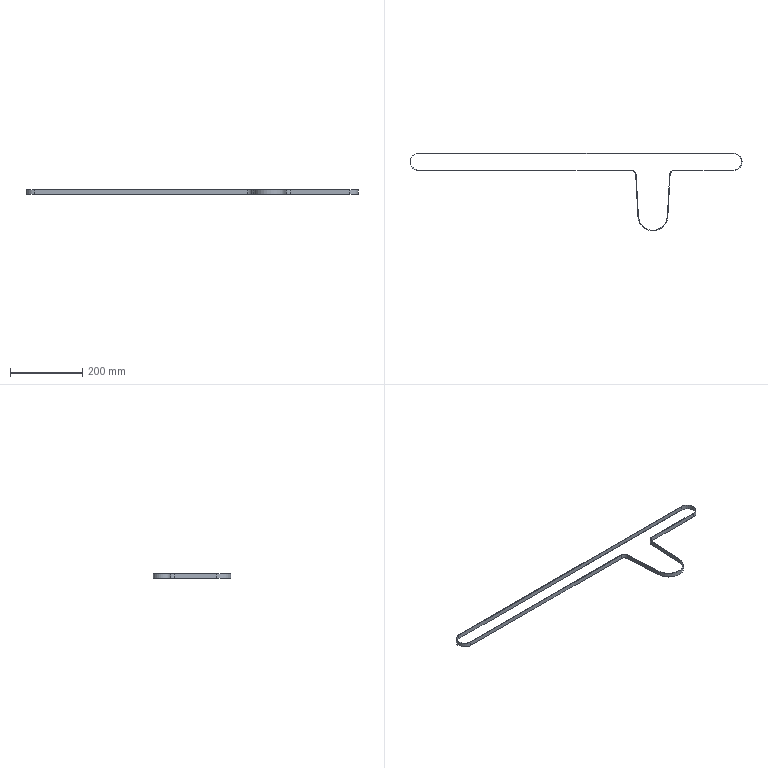Part | NX | features BREP 1 | 1 solid | 24 faces | box 917.4 x 214.1 x 12 mm | volume 31107 mm3 | cylinder 12 | plane 12 | commonest cylinder face diameters 45 x3 47.4 x3 25 x2 27.4 x2 80 x1 82.4 x1
STEP:
#1=CARTESIAN_POINT('',(764.214,8.857,-2.25));
#2=VERTEX_POINT('',#1);
#3=CARTESIAN_POINT('',(741.714,31.357,-2.25));
#4=VERTEX_POINT('',#3);
#5=CARTESIAN_POINT('',(741.714,8.857,-2.25));
#6=DIRECTION('',(0.,0.,1.));
#7=DIRECTION('',(-1.,0.,0.));
#8=AXIS2_PLACEMENT_3D('',#5,#6,#7);
#9=CIRCLE('',#8,22.5);
#10=EDGE_CURVE('',#2,#4,#9,.T.);
#11=ORIENTED_EDGE('',*,*,#10,.F.);
#12=CARTESIAN_POINT('',(764.214,8.857,9.75));
#13=VERTEX_POINT('',#12);
#14=CARTESIAN_POINT('',(764.214,8.857,-2.25));
#15=DIRECTION('',(0.,0.,1.));
#16=VECTOR('',#15,1000.);
#17=LINE('',#14,#16);
#18=EDGE_CURVE('',#2,#13,#17,.T.);
#19=ORIENTED_EDGE('',*,*,#18,.T.);
#20=CARTESIAN_POINT('',(741.714,31.357,9.75));
#21=VERTEX_POINT('',#20);
#22=CARTESIAN_POINT('',(741.714,8.857,9.75));
#23=DIRECTION('',(0.,0.,1.));
#24=DIRECTION('',(-1.,0.,0.));
#25=AXIS2_PLACEMENT_3D('',#22,#23,#24);
#26=CIRCLE('',#25,22.5);
#27=EDGE_CURVE('',#13,#21,#26,.T.);
#28=ORIENTED_EDGE('',*,*,#27,.T.);
#29=CARTESIAN_POINT('',(741.714,31.357,-2.25));
#30=DIRECTION('',(0.,0.,1.));
#31=VECTOR('',#30,1000.);
#32=LINE('',#29,#31);
#33=EDGE_CURVE('',#4,#21,#32,.T.);
#34=ORIENTED_EDGE('',*,*,#33,.F.);
#35=EDGE_LOOP('',(#11,#19,#28,#34));
#36=FACE_BOUND('',#35,.T.);
#37=CARTESIAN_POINT('',(741.714,8.857,-2.25));
#38=DIRECTION('',(0.,0.,1.));
#39=DIRECTION('',(1.,0.,0.));
#40=AXIS2_PLACEMENT_3D('',#37,#38,#39);
#41=CYLINDRICAL_SURFACE('',#40,22.5);
#42=ADVANCED_FACE('',(#36),#41,.F.);
#43=CARTESIAN_POINT('',(741.714,-14.843,-2.25));
#44=VERTEX_POINT('',#43);
#45=CARTESIAN_POINT('',(765.414,8.857,-2.25));
#46=VERTEX_POINT('',#45);
#47=CARTESIAN_POINT('',(741.714,8.857,-2.25));
#48=DIRECTION('',(0.,0.,1.));
#49=DIRECTION('',(1.,0.,0.));
#50=AXIS2_PLACEMENT_3D('',#47,#48,#49);
#51=CIRCLE('',#50,23.7);
#52=EDGE_CURVE('',#44,#46,#51,.T.);
#53=ORIENTED_EDGE('',*,*,#52,.T.);
#54=CARTESIAN_POINT('',(765.414,8.857,9.75));
#55=VERTEX_POINT('',#54);
#56=CARTESIAN_POINT('',(765.414,8.857,-2.25));
#57=DIRECTION('',(0.,0.,1.));
#58=VECTOR('',#57,1000.);
#59=LINE('',#56,#58);
#60=EDGE_CURVE('',#46,#55,#59,.T.);
#61=ORIENTED_EDGE('',*,*,#60,.T.);
#62=CARTESIAN_POINT('',(741.714,-14.843,9.75));
#63=VERTEX_POINT('',#62);
#64=CARTESIAN_POINT('',(741.714,8.857,9.75));
#65=DIRECTION('',(0.,0.,1.));
#66=DIRECTION('',(1.,0.,0.));
#67=AXIS2_PLACEMENT_3D('',#64,#65,#66);
#68=CIRCLE('',#67,23.7);
#69=EDGE_CURVE('',#63,#55,#68,.T.);
#70=ORIENTED_EDGE('',*,*,#69,.F.);
#71=CARTESIAN_POINT('',(741.714,-14.843,-2.25));
#72=DIRECTION('',(0.,0.,1.));
#73=VECTOR('',#72,1000.);
#74=LINE('',#71,#73);
#75=EDGE_CURVE('',#44,#63,#74,.T.);
#76=ORIENTED_EDGE('',*,*,#75,.F.);
#77=EDGE_LOOP('',(#53,#61,#70,#76));
#78=FACE_BOUND('',#77,.T.);
#79=CARTESIAN_POINT('',(741.714,8.857,-2.25));
#80=DIRECTION('',(0.,0.,1.));
#81=DIRECTION('',(1.,0.,0.));
#82=AXIS2_PLACEMENT_3D('',#79,#80,#81);
#83=CYLINDRICAL_SURFACE('',#82,23.7);
#84=ADVANCED_FACE('',(#78),#83,.T.);
#85=ORIENTED_EDGE('',*,*,#60,.F.);
#86=CARTESIAN_POINT('',(741.714,32.557,-2.25));
#87=VERTEX_POINT('',#86);
#88=CARTESIAN_POINT('',(741.714,8.857,-2.25));
#89=DIRECTION('',(0.,0.,1.));
#90=DIRECTION('',(1.,0.,0.));
#91=AXIS2_PLACEMENT_3D('',#88,#89,#90);
#92=CIRCLE('',#91,23.7);
#93=EDGE_CURVE('',#46,#87,#92,.T.);
#94=ORIENTED_EDGE('',*,*,#93,.T.);
#95=CARTESIAN_POINT('',(741.714,32.557,9.75));
#96=VERTEX_POINT('',#95);
#97=CARTESIAN_POINT('',(741.714,32.557,-2.25));
#98=DIRECTION('',(0.,0.,1.));
#99=VECTOR('',#98,1000.);
#100=LINE('',#97,#99);
#101=EDGE_CURVE('',#87,#96,#100,.T.);
#102=ORIENTED_EDGE('',*,*,#101,.T.);
#103=CARTESIAN_POINT('',(741.714,8.857,9.75));
#104=DIRECTION('',(0.,0.,1.));
#105=DIRECTION('',(1.,0.,0.));
#106=AXIS2_PLACEMENT_3D('',#103,#104,#105);
#107=CIRCLE('',#106,23.7);
#108=EDGE_CURVE('',#55,#96,#107,.T.);
#109=ORIENTED_EDGE('',*,*,#108,.F.);
#110=EDGE_LOOP('',(#85,#94,#102,#109));
#111=FACE_BOUND('',#110,.T.);
#112=CARTESIAN_POINT('',(741.714,8.857,-2.25));
#113=DIRECTION('',(0.,0.,1.));
#114=DIRECTION('',(1.,0.,0.));
#115=AXIS2_PLACEMENT_3D('',#112,#113,#114);
#116=CYLINDRICAL_SURFACE('',#115,23.7);
#117=ADVANCED_FACE('',(#111),#116,.T.);
#118=CARTESIAN_POINT('',(579.214,-14.843,9.75));
#119=VERTEX_POINT('',#118);
#120=CARTESIAN_POINT('',(579.214,-14.843,9.75));
#121=DIRECTION('',(1.,0.,0.));
#122=VECTOR('',#121,1000.);
#123=LINE('',#120,#122);
#124=EDGE_CURVE('',#119,#63,#123,.T.);
#125=ORIENTED_EDGE('',*,*,#124,.F.);
#126=CARTESIAN_POINT('',(579.214,-14.843,-2.25));
#127=VERTEX_POINT('',#126);
#128=CARTESIAN_POINT('',(579.214,-14.843,-2.25));
#129=DIRECTION('',(0.,0.,1.));
#130=VECTOR('',#129,1000.);
#131=LINE('',#128,#130);
#132=EDGE_CURVE('',#127,#119,#131,.T.);
#133=ORIENTED_EDGE('',*,*,#132,.F.);
#134=CARTESIAN_POINT('',(579.214,-14.843,-2.25));
#135=DIRECTION('',(1.,0.,0.));
#136=VECTOR('',#135,1000.);
#137=LINE('',#134,#136);
#138=EDGE_CURVE('',#127,#44,#137,.T.);
#139=ORIENTED_EDGE('',*,*,#138,.T.);
#140=ORIENTED_EDGE('',*,*,#75,.T.);
#141=EDGE_LOOP('',(#125,#133,#139,#140));
#142=FACE_BOUND('',#141,.T.);
#143=CARTESIAN_POINT('',(579.214,-14.843,-2.25));
#144=DIRECTION('',(0.,-1.,0.));
#145=DIRECTION('',(0.,0.,-1.));
#146=AXIS2_PLACEMENT_3D('',#143,#144,#145);
#147=PLANE('',#146);
#148=ADVANCED_FACE('',(#142),#147,.T.);
#149=CARTESIAN_POINT('',(566.733,-26.656,9.75));
#150=VERTEX_POINT('',#149);
#151=CARTESIAN_POINT('',(579.214,-27.343,9.75));
#152=DIRECTION('',(0.,0.,-1.));
#153=DIRECTION('',(-1.,0.,0.));
#154=AXIS2_PLACEMENT_3D('',#151,#152,#153);
#155=CIRCLE('',#154,12.5);
#156=EDGE_CURVE('',#150,#119,#155,.T.);
#157=ORIENTED_EDGE('',*,*,#156,.F.);
#158=CARTESIAN_POINT('',(566.733,-26.656,-2.25));
#159=VERTEX_POINT('',#158);
#160=CARTESIAN_POINT('',(566.733,-26.656,-2.25));
#161=DIRECTION('',(0.,0.,1.));
#162=VECTOR('',#161,1000.);
#163=LINE('',#160,#162);
#164=EDGE_CURVE('',#159,#150,#163,.T.);
#165=ORIENTED_EDGE('',*,*,#164,.F.);
#166=CARTESIAN_POINT('',(579.214,-27.343,-2.25));
#167=DIRECTION('',(0.,0.,-1.));
#168=DIRECTION('',(-1.,0.,0.));
#169=AXIS2_PLACEMENT_3D('',#166,#167,#168);
#170=CIRCLE('',#169,12.5);
#171=EDGE_CURVE('',#159,#127,#170,.T.);
#172=ORIENTED_EDGE('',*,*,#171,.T.);
#173=ORIENTED_EDGE('',*,*,#132,.T.);
#174=EDGE_LOOP('',(#157,#165,#172,#173));
#175=FACE_BOUND('',#174,.T.);
#176=CARTESIAN_POINT('',(579.214,-27.343,-2.25));
#177=DIRECTION('',(0.,0.,1.));
#178=DIRECTION('',(1.,0.,0.));
#179=AXIS2_PLACEMENT_3D('',#176,#177,#178);
#180=CYLINDRICAL_SURFACE('',#179,12.5);
#181=ADVANCED_FACE('',(#175),#180,.F.);
#182=CARTESIAN_POINT('',(560.352,-142.607,9.75));
#183=VERTEX_POINT('',#182);
#184=CARTESIAN_POINT('',(560.352,-142.607,9.75));
#185=DIRECTION('',(0.05495,0.9985,0.));
#186=VECTOR('',#185,1000.);
#187=LINE('',#184,#186);
#188=EDGE_CURVE('',#183,#150,#187,.T.);
#189=ORIENTED_EDGE('',*,*,#188,.F.);
#190=CARTESIAN_POINT('',(560.352,-142.607,-2.25));
#191=VERTEX_POINT('',#190);
#192=CARTESIAN_POINT('',(560.352,-142.607,-2.25));
#193=DIRECTION('',(0.,0.,1.));
#194=VECTOR('',#193,1000.);
#195=LINE('',#192,#194);
#196=EDGE_CURVE('',#191,#183,#195,.T.);
#197=ORIENTED_EDGE('',*,*,#196,.F.);
#198=CARTESIAN_POINT('',(560.352,-142.607,-2.25));
#199=DIRECTION('',(0.05495,0.9985,0.));
#200=VECTOR('',#199,1000.);
#201=LINE('',#198,#200);
#202=EDGE_CURVE('',#191,#159,#201,.T.);
#203=ORIENTED_EDGE('',*,*,#202,.T.);
#204=ORIENTED_EDGE('',*,*,#164,.T.);
#205=EDGE_LOOP('',(#189,#197,#203,#204));
#206=FACE_BOUND('',#205,.T.);
#207=CARTESIAN_POINT('',(560.352,-142.607,-2.25));
#208=DIRECTION('',(0.9985,-0.05495,0.));
#209=DIRECTION('',(0.,0.,-1.));
#210=AXIS2_PLACEMENT_3D('',#207,#208,#209);
#211=PLANE('',#210);
#212=ADVANCED_FACE('',(#206),#211,.T.);
#213=CARTESIAN_POINT('',(478.077,-142.607,9.75));
#214=VERTEX_POINT('',#213);
#215=CARTESIAN_POINT('',(519.214,-140.343,9.75));
#216=DIRECTION('',(0.,0.,1.));
#217=DIRECTION('',(1.,0.,0.));
#218=AXIS2_PLACEMENT_3D('',#215,#216,#217);
#219=CIRCLE('',#218,41.2);
#220=EDGE_CURVE('',#214,#183,#219,.T.);
#221=ORIENTED_EDGE('',*,*,#220,.F.);
#222=CARTESIAN_POINT('',(478.077,-142.607,-2.25));
#223=VERTEX_POINT('',#222);
#224=CARTESIAN_POINT('',(478.077,-142.607,-2.25));
#225=DIRECTION('',(0.,0.,1.));
#226=VECTOR('',#225,1000.);
#227=LINE('',#224,#226);
#228=EDGE_CURVE('',#223,#214,#227,.T.);
#229=ORIENTED_EDGE('',*,*,#228,.F.);
#230=CARTESIAN_POINT('',(519.214,-140.343,-2.25));
#231=DIRECTION('',(0.,0.,1.));
#232=DIRECTION('',(1.,0.,0.));
#233=AXIS2_PLACEMENT_3D('',#230,#231,#232);
#234=CIRCLE('',#233,41.2);
#235=EDGE_CURVE('',#223,#191,#234,.T.);
#236=ORIENTED_EDGE('',*,*,#235,.T.);
#237=ORIENTED_EDGE('',*,*,#196,.T.);
#238=EDGE_LOOP('',(#221,#229,#236,#237));
#239=FACE_BOUND('',#238,.T.);
#240=CARTESIAN_POINT('',(519.214,-140.343,-2.25));
#241=DIRECTION('',(0.,0.,1.));
#242=DIRECTION('',(1.,0.,0.));
#243=AXIS2_PLACEMENT_3D('',#240,#241,#242);
#244=CYLINDRICAL_SURFACE('',#243,41.2);
#245=ADVANCED_FACE('',(#239),#244,.T.);
#246=CARTESIAN_POINT('',(471.695,-26.656,9.75));
#247=VERTEX_POINT('',#246);
#248=CARTESIAN_POINT('',(471.695,-26.656,9.75));
#249=DIRECTION('',(0.05495,-0.9985,0.));
#250=VECTOR('',#249,1000.);
#251=LINE('',#248,#250);
#252=EDGE_CURVE('',#247,#214,#251,.T.);
#253=ORIENTED_EDGE('',*,*,#252,.F.);
#254=CARTESIAN_POINT('',(471.695,-26.656,-2.25));
#255=VERTEX_POINT('',#254);
#256=CARTESIAN_POINT('',(471.695,-26.656,-2.25));
#257=DIRECTION('',(0.,0.,1.));
#258=VECTOR('',#257,1000.);
#259=LINE('',#256,#258);
#260=EDGE_CURVE('',#255,#247,#259,.T.);
#261=ORIENTED_EDGE('',*,*,#260,.F.);
#262=CARTESIAN_POINT('',(471.695,-26.656,-2.25));
#263=DIRECTION('',(0.05495,-0.9985,0.));
#264=VECTOR('',#263,1000.);
#265=LINE('',#262,#264);
#266=EDGE_CURVE('',#255,#223,#265,.T.);
#267=ORIENTED_EDGE('',*,*,#266,.T.);
#268=ORIENTED_EDGE('',*,*,#228,.T.);
#269=EDGE_LOOP('',(#253,#261,#267,#268));
#270=FACE_BOUND('',#269,.T.);
#271=CARTESIAN_POINT('',(471.695,-26.656,-2.25));
#272=DIRECTION('',(-0.9985,-0.05495,0.));
#273=DIRECTION('',(-0.05495,0.9985,0.));
#274=AXIS2_PLACEMENT_3D('',#271,#272,#273);
#275=PLANE('',#274);
#276=ADVANCED_FACE('',(#270),#275,.T.);
#277=CARTESIAN_POINT('',(459.214,-14.843,9.75));
#278=VERTEX_POINT('',#277);
#279=CARTESIAN_POINT('',(459.214,-27.343,9.75));
#280=DIRECTION('',(0.,0.,-1.));
#281=DIRECTION('',(-1.,0.,0.));
#282=AXIS2_PLACEMENT_3D('',#279,#280,#281);
#283=CIRCLE('',#282,12.5);
#284=EDGE_CURVE('',#278,#247,#283,.T.);
#285=ORIENTED_EDGE('',*,*,#284,.F.);
#286=CARTESIAN_POINT('',(459.214,-14.843,-2.25));
#287=VERTEX_POINT('',#286);
#288=CARTESIAN_POINT('',(459.214,-14.843,-2.25));
#289=DIRECTION('',(0.,0.,1.));
#290=VECTOR('',#289,1000.);
#291=LINE('',#288,#290);
#292=EDGE_CURVE('',#287,#278,#291,.T.);
#293=ORIENTED_EDGE('',*,*,#292,.F.);
#294=CARTESIAN_POINT('',(459.214,-27.343,-2.25));
#295=DIRECTION('',(0.,0.,-1.));
#296=DIRECTION('',(-1.,0.,0.));
#297=AXIS2_PLACEMENT_3D('',#294,#295,#296);
#298=CIRCLE('',#297,12.5);
#299=EDGE_CURVE('',#287,#255,#298,.T.);
#300=ORIENTED_EDGE('',*,*,#299,.T.);
#301=ORIENTED_EDGE('',*,*,#260,.T.);
#302=EDGE_LOOP('',(#285,#293,#300,#301));
#303=FACE_BOUND('',#302,.T.);
#304=CARTESIAN_POINT('',(459.214,-27.343,-2.25));
#305=DIRECTION('',(0.,0.,1.));
#306=DIRECTION('',(1.,0.,0.));
#307=AXIS2_PLACEMENT_3D('',#304,#305,#306);
#308=CYLINDRICAL_SURFACE('',#307,12.5);
#309=ADVANCED_FACE('',(#303),#308,.F.);
#310=CARTESIAN_POINT('',(-128.286,-14.843,9.75));
#311=VERTEX_POINT('',#310);
#312=CARTESIAN_POINT('',(-128.286,-14.843,9.75));
#313=DIRECTION('',(1.,0.,0.));
#314=VECTOR('',#313,1000.);
#315=LINE('',#312,#314);
#316=EDGE_CURVE('',#311,#278,#315,.T.);
#317=ORIENTED_EDGE('',*,*,#316,.F.);
#318=CARTESIAN_POINT('',(-128.286,-14.843,-2.25));
#319=VERTEX_POINT('',#318);
#320=CARTESIAN_POINT('',(-128.286,-14.843,-2.25));
#321=DIRECTION('',(0.,0.,1.));
#322=VECTOR('',#321,1000.);
#323=LINE('',#320,#322);
#324=EDGE_CURVE('',#319,#311,#323,.T.);
#325=ORIENTED_EDGE('',*,*,#324,.F.);
#326=CARTESIAN_POINT('',(-128.286,-14.843,-2.25));
#327=DIRECTION('',(1.,0.,0.));
#328=VECTOR('',#327,1000.);
#329=LINE('',#326,#328);
#330=EDGE_CURVE('',#319,#287,#329,.T.);
#331=ORIENTED_EDGE('',*,*,#330,.T.);
#332=ORIENTED_EDGE('',*,*,#292,.T.);
#333=EDGE_LOOP('',(#317,#325,#331,#332));
#334=FACE_BOUND('',#333,.T.);
#335=CARTESIAN_POINT('',(-128.286,-14.843,-2.25));
#336=DIRECTION('',(0.,-1.,0.));
#337=DIRECTION('',(-1.,0.,0.));
#338=AXIS2_PLACEMENT_3D('',#335,#336,#337);
#339=PLANE('',#338);
#340=ADVANCED_FACE('',(#334),#339,.T.);
#341=CARTESIAN_POINT('',(-128.286,32.557,9.75));
#342=VERTEX_POINT('',#341);
#343=CARTESIAN_POINT('',(-128.286,8.857,9.75));
#344=DIRECTION('',(0.,0.,1.));
#345=DIRECTION('',(1.,0.,0.));
#346=AXIS2_PLACEMENT_3D('',#343,#344,#345);
#347=CIRCLE('',#346,23.7);
#348=EDGE_CURVE('',#342,#311,#347,.T.);
#349=ORIENTED_EDGE('',*,*,#348,.F.);
#350=CARTESIAN_POINT('',(-128.286,32.557,-2.25));
#351=VERTEX_POINT('',#350);
#352=CARTESIAN_POINT('',(-128.286,32.557,-2.25));
#353=DIRECTION('',(0.,0.,1.));
#354=VECTOR('',#353,1000.);
#355=LINE('',#352,#354);
#356=EDGE_CURVE('',#351,#342,#355,.T.);
#357=ORIENTED_EDGE('',*,*,#356,.F.);
#358=CARTESIAN_POINT('',(-128.286,8.857,-2.25));
#359=DIRECTION('',(0.,0.,1.));
#360=DIRECTION('',(1.,0.,0.));
#361=AXIS2_PLACEMENT_3D('',#358,#359,#360);
#362=CIRCLE('',#361,23.7);
#363=EDGE_CURVE('',#351,#319,#362,.T.);
#364=ORIENTED_EDGE('',*,*,#363,.T.);
#365=ORIENTED_EDGE('',*,*,#324,.T.);
#366=EDGE_LOOP('',(#349,#357,#364,#365));
#367=FACE_BOUND('',#366,.T.);
#368=CARTESIAN_POINT('',(-128.286,8.857,-2.25));
#369=DIRECTION('',(0.,0.,1.));
#370=DIRECTION('',(1.,0.,0.));
#371=AXIS2_PLACEMENT_3D('',#368,#369,#370);
#372=CYLINDRICAL_SURFACE('',#371,23.7);
#373=ADVANCED_FACE('',(#367),#372,.T.);
#374=CARTESIAN_POINT('',(741.714,32.557,9.75));
#375=DIRECTION('',(-1.,0.,0.));
#376=VECTOR('',#375,1000.);
#377=LINE('',#374,#376);
#378=EDGE_CURVE('',#96,#342,#377,.T.);
#379=ORIENTED_EDGE('',*,*,#378,.F.);
#380=ORIENTED_EDGE('',*,*,#101,.F.);
#381=CARTESIAN_POINT('',(741.714,32.557,-2.25));
#382=DIRECTION('',(-1.,0.,0.));
#383=VECTOR('',#382,1000.);
#384=LINE('',#381,#383);
#385=EDGE_CURVE('',#87,#351,#384,.T.);
#386=ORIENTED_EDGE('',*,*,#385,.T.);
#387=ORIENTED_EDGE('',*,*,#356,.T.);
#388=EDGE_LOOP('',(#379,#380,#386,#387));
#389=FACE_BOUND('',#388,.T.);
#390=CARTESIAN_POINT('',(741.714,32.557,-2.25));
#391=DIRECTION('',(0.,1.,0.));
#392=DIRECTION('',(1.,0.,0.));
#393=AXIS2_PLACEMENT_3D('',#390,#391,#392);
#394=PLANE('',#393);
#395=ADVANCED_FACE('',(#389),#394,.T.);
#396=ORIENTED_EDGE('',*,*,#52,.F.);
#397=ORIENTED_EDGE('',*,*,#138,.F.);
#398=ORIENTED_EDGE('',*,*,#171,.F.);
#399=ORIENTED_EDGE('',*,*,#202,.F.);
#400=ORIENTED_EDGE('',*,*,#235,.F.);
#401=ORIENTED_EDGE('',*,*,#266,.F.);
#402=ORIENTED_EDGE('',*,*,#299,.F.);
#403=ORIENTED_EDGE('',*,*,#330,.F.);
#404=ORIENTED_EDGE('',*,*,#363,.F.);
#405=ORIENTED_EDGE('',*,*,#385,.F.);
#406=ORIENTED_EDGE('',*,*,#93,.F.);
#407=EDGE_LOOP('',(#396,#397,#398,#399,#400,#401,#402,#403,#404,#405,#406));
#408=FACE_BOUND('',#407,.T.);
#409=CARTESIAN_POINT('',(472.894,-26.59,-2.25));
#410=VERTEX_POINT('',#409);
#411=CARTESIAN_POINT('',(479.275,-142.541,-2.25));
#412=VERTEX_POINT('',#411);
#413=CARTESIAN_POINT('',(479.275,-142.541,-2.25));
#414=DIRECTION('',(0.05495,-0.9985,0.));
#415=VECTOR('',#414,1000.);
#416=LINE('',#413,#415);
#417=EDGE_CURVE('',#410,#412,#416,.T.);
#418=ORIENTED_EDGE('',*,*,#417,.T.);
#419=CARTESIAN_POINT('',(559.154,-142.541,-2.25));
#420=VERTEX_POINT('',#419);
#421=CARTESIAN_POINT('',(519.214,-140.343,-2.25));
#422=DIRECTION('',(0.,0.,1.));
#423=DIRECTION('',(-1.,0.,0.));
#424=AXIS2_PLACEMENT_3D('',#421,#422,#423);
#425=CIRCLE('',#424,40.);
#426=EDGE_CURVE('',#412,#420,#425,.T.);
#427=ORIENTED_EDGE('',*,*,#426,.T.);
#428=CARTESIAN_POINT('',(565.535,-26.59,-2.25));
#429=VERTEX_POINT('',#428);
#430=CARTESIAN_POINT('',(565.535,-26.59,-2.25));
#431=DIRECTION('',(0.05495,0.9985,0.));
#432=VECTOR('',#431,1000.);
#433=LINE('',#430,#432);
#434=EDGE_CURVE('',#420,#429,#433,.T.);
#435=ORIENTED_EDGE('',*,*,#434,.T.);
#436=CARTESIAN_POINT('',(579.214,-13.643,-2.25));
#437=VERTEX_POINT('',#436);
#438=CARTESIAN_POINT('',(579.214,-27.343,-2.25));
#439=DIRECTION('',(0.,0.,-1.));
#440=DIRECTION('',(1.,0.,0.));
#441=AXIS2_PLACEMENT_3D('',#438,#439,#440);
#442=CIRCLE('',#441,13.7);
#443=EDGE_CURVE('',#429,#437,#442,.T.);
#444=ORIENTED_EDGE('',*,*,#443,.T.);
#445=CARTESIAN_POINT('',(741.714,-13.643,-2.25));
#446=VERTEX_POINT('',#445);
#447=CARTESIAN_POINT('',(741.714,-13.643,-2.25));
#448=DIRECTION('',(1.,0.,0.));
#449=VECTOR('',#448,1000.);
#450=LINE('',#447,#449);
#451=EDGE_CURVE('',#437,#446,#450,.T.);
#452=ORIENTED_EDGE('',*,*,#451,.T.);
#453=CARTESIAN_POINT('',(741.714,8.857,-2.25));
#454=DIRECTION('',(0.,0.,1.));
#455=DIRECTION('',(-1.,0.,0.));
#456=AXIS2_PLACEMENT_3D('',#453,#454,#455);
#457=CIRCLE('',#456,22.5);
#458=EDGE_CURVE('',#446,#2,#457,.T.);
#459=ORIENTED_EDGE('',*,*,#458,.T.);
#460=ORIENTED_EDGE('',*,*,#10,.T.);
#461=CARTESIAN_POINT('',(-128.286,31.357,-2.25));
#462=VERTEX_POINT('',#461);
#463=CARTESIAN_POINT('',(-128.286,31.357,-2.25));
#464=DIRECTION('',(-1.,0.,0.));
#465=VECTOR('',#464,1000.);
#466=LINE('',#463,#465);
#467=EDGE_CURVE('',#4,#462,#466,.T.);
#468=ORIENTED_EDGE('',*,*,#467,.T.);
#469=CARTESIAN_POINT('',(-128.286,-13.643,-2.25));
#470=VERTEX_POINT('',#469);
#471=CARTESIAN_POINT('',(-128.286,8.857,-2.25));
#472=DIRECTION('',(0.,0.,1.));
#473=DIRECTION('',(-1.,0.,0.));
#474=AXIS2_PLACEMENT_3D('',#471,#472,#473);
#475=CIRCLE('',#474,22.5);
#476=EDGE_CURVE('',#462,#470,#475,.T.);
#477=ORIENTED_EDGE('',*,*,#476,.T.);
#478=CARTESIAN_POINT('',(459.214,-13.643,-2.25));
#479=VERTEX_POINT('',#478);
#480=CARTESIAN_POINT('',(459.214,-13.643,-2.25));
#481=DIRECTION('',(1.,0.,0.));
#482=VECTOR('',#481,1000.);
#483=LINE('',#480,#482);
#484=EDGE_CURVE('',#470,#479,#483,.T.);
#485=ORIENTED_EDGE('',*,*,#484,.T.);
#486=CARTESIAN_POINT('',(459.214,-27.343,-2.25));
#487=DIRECTION('',(0.,0.,-1.));
#488=DIRECTION('',(1.,0.,0.));
#489=AXIS2_PLACEMENT_3D('',#486,#487,#488);
#490=CIRCLE('',#489,13.7);
#491=EDGE_CURVE('',#479,#410,#490,.T.);
#492=ORIENTED_EDGE('',*,*,#491,.T.);
#493=EDGE_LOOP('',(#418,#427,#435,#444,#452,#459,#460,#468,#477,#485,#492));
#494=FACE_BOUND('',#493,.T.);
#495=CARTESIAN_POINT('',(741.714,8.857,-2.25));
#496=DIRECTION('',(0.,0.,1.));
#497=DIRECTION('',(1.,0.,0.));
#498=AXIS2_PLACEMENT_3D('',#495,#496,#497);
#499=PLANE('',#498);
#500=ADVANCED_FACE('',(#408,#494),#499,.F.);
#501=ORIENTED_EDGE('',*,*,#69,.T.);
#502=ORIENTED_EDGE('',*,*,#108,.T.);
#503=ORIENTED_EDGE('',*,*,#378,.T.);
#504=ORIENTED_EDGE('',*,*,#348,.T.);
#505=ORIENTED_EDGE('',*,*,#316,.T.);
#506=ORIENTED_EDGE('',*,*,#284,.T.);
#507=ORIENTED_EDGE('',*,*,#252,.T.);
#508=ORIENTED_EDGE('',*,*,#220,.T.);
#509=ORIENTED_EDGE('',*,*,#188,.T.);
#510=ORIENTED_EDGE('',*,*,#156,.T.);
#511=ORIENTED_EDGE('',*,*,#124,.T.);
#512=EDGE_LOOP('',(#501,#502,#503,#504,#505,#506,#507,#508,#509,#510,#511));
#513=FACE_BOUND('',#512,.T.);
#514=CARTESIAN_POINT('',(479.275,-142.541,9.75));
#515=VERTEX_POINT('',#514);
#516=CARTESIAN_POINT('',(559.154,-142.541,9.75));
#517=VERTEX_POINT('',#516);
#518=CARTESIAN_POINT('',(519.214,-140.343,9.75));
#519=DIRECTION('',(0.,0.,1.));
#520=DIRECTION('',(-1.,0.,0.));
#521=AXIS2_PLACEMENT_3D('',#518,#519,#520);
#522=CIRCLE('',#521,40.);
#523=EDGE_CURVE('',#515,#517,#522,.T.);
#524=ORIENTED_EDGE('',*,*,#523,.F.);
#525=CARTESIAN_POINT('',(472.894,-26.59,9.75));
#526=VERTEX_POINT('',#525);
#527=CARTESIAN_POINT('',(479.275,-142.541,9.75));
#528=DIRECTION('',(0.05495,-0.9985,0.));
#529=VECTOR('',#528,1000.);
#530=LINE('',#527,#529);
#531=EDGE_CURVE('',#526,#515,#530,.T.);
#532=ORIENTED_EDGE('',*,*,#531,.F.);
#533=CARTESIAN_POINT('',(459.214,-13.643,9.75));
#534=VERTEX_POINT('',#533);
#535=CARTESIAN_POINT('',(459.214,-27.343,9.75));
#536=DIRECTION('',(0.,0.,-1.));
#537=DIRECTION('',(1.,0.,0.));
#538=AXIS2_PLACEMENT_3D('',#535,#536,#537);
#539=CIRCLE('',#538,13.7);
#540=EDGE_CURVE('',#534,#526,#539,.T.);
#541=ORIENTED_EDGE('',*,*,#540,.F.);
#542=CARTESIAN_POINT('',(-128.286,-13.643,9.75));
#543=VERTEX_POINT('',#542);
#544=CARTESIAN_POINT('',(459.214,-13.643,9.75));
#545=DIRECTION('',(1.,0.,0.));
#546=VECTOR('',#545,1000.);
#547=LINE('',#544,#546);
#548=EDGE_CURVE('',#543,#534,#547,.T.);
#549=ORIENTED_EDGE('',*,*,#548,.F.);
#550=CARTESIAN_POINT('',(-128.286,31.357,9.75));
#551=VERTEX_POINT('',#550);
#552=CARTESIAN_POINT('',(-128.286,8.857,9.75));
#553=DIRECTION('',(0.,0.,1.));
#554=DIRECTION('',(-1.,0.,0.));
#555=AXIS2_PLACEMENT_3D('',#552,#553,#554);
#556=CIRCLE('',#555,22.5);
#557=EDGE_CURVE('',#551,#543,#556,.T.);
#558=ORIENTED_EDGE('',*,*,#557,.F.);
#559=CARTESIAN_POINT('',(-128.286,31.357,9.75));
#560=DIRECTION('',(-1.,0.,0.));
#561=VECTOR('',#560,1000.);
#562=LINE('',#559,#561);
#563=EDGE_CURVE('',#21,#551,#562,.T.);
#564=ORIENTED_EDGE('',*,*,#563,.F.);
#565=ORIENTED_EDGE('',*,*,#27,.F.);
#566=CARTESIAN_POINT('',(741.714,-13.643,9.75));
#567=VERTEX_POINT('',#566);
#568=CARTESIAN_POINT('',(741.714,8.857,9.75));
#569=DIRECTION('',(0.,0.,1.));
#570=DIRECTION('',(-1.,0.,0.));
#571=AXIS2_PLACEMENT_3D('',#568,#569,#570);
#572=CIRCLE('',#571,22.5);
#573=EDGE_CURVE('',#567,#13,#572,.T.);
#574=ORIENTED_EDGE('',*,*,#573,.F.);
#575=CARTESIAN_POINT('',(579.214,-13.643,9.75));
#576=VERTEX_POINT('',#575);
#577=CARTESIAN_POINT('',(741.714,-13.643,9.75));
#578=DIRECTION('',(1.,0.,0.));
#579=VECTOR('',#578,1000.);
#580=LINE('',#577,#579);
#581=EDGE_CURVE('',#576,#567,#580,.T.);
#582=ORIENTED_EDGE('',*,*,#581,.F.);
#583=CARTESIAN_POINT('',(565.535,-26.59,9.75));
#584=VERTEX_POINT('',#583);
#585=CARTESIAN_POINT('',(579.214,-27.343,9.75));
#586=DIRECTION('',(0.,0.,-1.));
#587=DIRECTION('',(1.,0.,0.));
#588=AXIS2_PLACEMENT_3D('',#585,#586,#587);
#589=CIRCLE('',#588,13.7);
#590=EDGE_CURVE('',#584,#576,#589,.T.);
#591=ORIENTED_EDGE('',*,*,#590,.F.);
#592=CARTESIAN_POINT('',(565.535,-26.59,9.75));
#593=DIRECTION('',(0.05495,0.9985,0.));
#594=VECTOR('',#593,1000.);
#595=LINE('',#592,#594);
#596=EDGE_CURVE('',#517,#584,#595,.T.);
#597=ORIENTED_EDGE('',*,*,#596,.F.);
#598=EDGE_LOOP('',(#524,#532,#541,#549,#558,#564,#565,#574,#582,#591,#597));
#599=FACE_BOUND('',#598,.T.);
#600=CARTESIAN_POINT('',(741.714,8.857,9.75));
#601=DIRECTION('',(0.,0.,1.));
#602=DIRECTION('',(1.,0.,0.));
#603=AXIS2_PLACEMENT_3D('',#600,#601,#602);
#604=PLANE('',#603);
#605=ADVANCED_FACE('',(#513,#599),#604,.T.);
#606=ORIENTED_EDGE('',*,*,#523,.T.);
#607=CARTESIAN_POINT('',(559.154,-142.541,-2.25));
#608=DIRECTION('',(0.,0.,1.));
#609=VECTOR('',#608,1000.);
#610=LINE('',#607,#609);
#611=EDGE_CURVE('',#420,#517,#610,.T.);
#612=ORIENTED_EDGE('',*,*,#611,.F.);
#613=ORIENTED_EDGE('',*,*,#426,.F.);
#614=CARTESIAN_POINT('',(479.275,-142.541,-2.25));
#615=DIRECTION('',(0.,0.,1.));
#616=VECTOR('',#615,1000.);
#617=LINE('',#614,#616);
#618=EDGE_CURVE('',#412,#515,#617,.T.);
#619=ORIENTED_EDGE('',*,*,#618,.T.);
#620=EDGE_LOOP('',(#606,#612,#613,#619));
#621=FACE_BOUND('',#620,.T.);
#622=CARTESIAN_POINT('',(519.214,-140.343,-2.25));
#623=DIRECTION('',(0.,0.,1.));
#624=DIRECTION('',(1.,0.,0.));
#625=AXIS2_PLACEMENT_3D('',#622,#623,#624);
#626=CYLINDRICAL_SURFACE('',#625,40.);
#627=ADVANCED_FACE('',(#621),#626,.F.);
#628=ORIENTED_EDGE('',*,*,#531,.T.);
#629=ORIENTED_EDGE('',*,*,#618,.F.);
#630=ORIENTED_EDGE('',*,*,#417,.F.);
#631=CARTESIAN_POINT('',(472.894,-26.59,-2.25));
#632=DIRECTION('',(0.,0.,1.));
#633=VECTOR('',#632,1000.);
#634=LINE('',#631,#633);
#635=EDGE_CURVE('',#410,#526,#634,.T.);
#636=ORIENTED_EDGE('',*,*,#635,.T.);
#637=EDGE_LOOP('',(#628,#629,#630,#636));
#638=FACE_BOUND('',#637,.T.);
#639=CARTESIAN_POINT('',(479.275,-142.541,-2.25));
#640=DIRECTION('',(-0.9985,-0.05495,0.));
#641=DIRECTION('',(-0.05495,0.9985,0.));
#642=AXIS2_PLACEMENT_3D('',#639,#640,#641);
#643=PLANE('',#642);
#644=ADVANCED_FACE('',(#638),#643,.F.);
#645=ORIENTED_EDGE('',*,*,#540,.T.);
#646=ORIENTED_EDGE('',*,*,#635,.F.);
#647=ORIENTED_EDGE('',*,*,#491,.F.);
#648=CARTESIAN_POINT('',(459.214,-13.643,-2.25));
#649=DIRECTION('',(0.,0.,1.));
#650=VECTOR('',#649,1000.);
#651=LINE('',#648,#650);
#652=EDGE_CURVE('',#479,#534,#651,.T.);
#653=ORIENTED_EDGE('',*,*,#652,.T.);
#654=EDGE_LOOP('',(#645,#646,#647,#653));
#655=FACE_BOUND('',#654,.T.);
#656=CARTESIAN_POINT('',(459.214,-27.343,-2.25));
#657=DIRECTION('',(0.,0.,1.));
#658=DIRECTION('',(1.,0.,0.));
#659=AXIS2_PLACEMENT_3D('',#656,#657,#658);
#660=CYLINDRICAL_SURFACE('',#659,13.7);
#661=ADVANCED_FACE('',(#655),#660,.T.);
#662=ORIENTED_EDGE('',*,*,#548,.T.);
#663=ORIENTED_EDGE('',*,*,#652,.F.);
#664=ORIENTED_EDGE('',*,*,#484,.F.);
#665=CARTESIAN_POINT('',(-128.286,-13.643,-2.25));
#666=DIRECTION('',(0.,0.,1.));
#667=VECTOR('',#666,1000.);
#668=LINE('',#665,#667);
#669=EDGE_CURVE('',#470,#543,#668,.T.);
#670=ORIENTED_EDGE('',*,*,#669,.T.);
#671=EDGE_LOOP('',(#662,#663,#664,#670));
#672=FACE_BOUND('',#671,.T.);
#673=CARTESIAN_POINT('',(459.214,-13.643,-2.25));
#674=DIRECTION('',(0.,-1.,0.));
#675=DIRECTION('',(0.,0.,-1.));
#676=AXIS2_PLACEMENT_3D('',#673,#674,#675);
#677=PLANE('',#676);
#678=ADVANCED_FACE('',(#672),#677,.F.);
#679=ORIENTED_EDGE('',*,*,#557,.T.);
#680=ORIENTED_EDGE('',*,*,#669,.F.);
#681=ORIENTED_EDGE('',*,*,#476,.F.);
#682=CARTESIAN_POINT('',(-128.286,31.357,-2.25));
#683=DIRECTION('',(0.,0.,1.));
#684=VECTOR('',#683,1000.);
#685=LINE('',#682,#684);
#686=EDGE_CURVE('',#462,#551,#685,.T.);
#687=ORIENTED_EDGE('',*,*,#686,.T.);
#688=EDGE_LOOP('',(#679,#680,#681,#687));
#689=FACE_BOUND('',#688,.T.);
#690=CARTESIAN_POINT('',(-128.286,8.857,-2.25));
#691=DIRECTION('',(0.,0.,1.));
#692=DIRECTION('',(1.,0.,0.));
#693=AXIS2_PLACEMENT_3D('',#690,#691,#692);
#694=CYLINDRICAL_SURFACE('',#693,22.5);
#695=ADVANCED_FACE('',(#689),#694,.F.);
#696=ORIENTED_EDGE('',*,*,#563,.T.);
#697=ORIENTED_EDGE('',*,*,#686,.F.);
#698=ORIENTED_EDGE('',*,*,#467,.F.);
#699=ORIENTED_EDGE('',*,*,#33,.T.);
#700=EDGE_LOOP('',(#696,#697,#698,#699));
#701=FACE_BOUND('',#700,.T.);
#702=CARTESIAN_POINT('',(-128.286,31.357,-2.25));
#703=DIRECTION('',(0.,1.,0.));
#704=DIRECTION('',(1.,0.,0.));
#705=AXIS2_PLACEMENT_3D('',#702,#703,#704);
#706=PLANE('',#705);
#707=ADVANCED_FACE('',(#701),#706,.F.);
#708=ORIENTED_EDGE('',*,*,#18,.F.);
#709=ORIENTED_EDGE('',*,*,#458,.F.);
#710=CARTESIAN_POINT('',(741.714,-13.643,-2.25));
#711=DIRECTION('',(0.,0.,1.));
#712=VECTOR('',#711,1000.);
#713=LINE('',#710,#712);
#714=EDGE_CURVE('',#446,#567,#713,.T.);
#715=ORIENTED_EDGE('',*,*,#714,.T.);
#716=ORIENTED_EDGE('',*,*,#573,.T.);
#717=EDGE_LOOP('',(#708,#709,#715,#716));
#718=FACE_BOUND('',#717,.T.);
#719=CARTESIAN_POINT('',(741.714,8.857,-2.25));
#720=DIRECTION('',(0.,0.,1.));
#721=DIRECTION('',(1.,0.,0.));
#722=AXIS2_PLACEMENT_3D('',#719,#720,#721);
#723=CYLINDRICAL_SURFACE('',#722,22.5);
#724=ADVANCED_FACE('',(#718),#723,.F.);
#725=ORIENTED_EDGE('',*,*,#581,.T.);
#726=ORIENTED_EDGE('',*,*,#714,.F.);
#727=ORIENTED_EDGE('',*,*,#451,.F.);
#728=CARTESIAN_POINT('',(579.214,-13.643,-2.25));
#729=DIRECTION('',(0.,0.,1.));
#730=VECTOR('',#729,1000.);
#731=LINE('',#728,#730);
#732=EDGE_CURVE('',#437,#576,#731,.T.);
#733=ORIENTED_EDGE('',*,*,#732,.T.);
#734=EDGE_LOOP('',(#725,#726,#727,#733));
#735=FACE_BOUND('',#734,.T.);
#736=CARTESIAN_POINT('',(741.714,-13.643,-2.25));
#737=DIRECTION('',(0.,-1.,0.));
#738=DIRECTION('',(0.,0.,-1.));
#739=AXIS2_PLACEMENT_3D('',#736,#737,#738);
#740=PLANE('',#739);
#741=ADVANCED_FACE('',(#735),#740,.F.);
#742=ORIENTED_EDGE('',*,*,#590,.T.);
#743=ORIENTED_EDGE('',*,*,#732,.F.);
#744=ORIENTED_EDGE('',*,*,#443,.F.);
#745=CARTESIAN_POINT('',(565.535,-26.59,-2.25));
#746=DIRECTION('',(0.,0.,1.));
#747=VECTOR('',#746,1000.);
#748=LINE('',#745,#747);
#749=EDGE_CURVE('',#429,#584,#748,.T.);
#750=ORIENTED_EDGE('',*,*,#749,.T.);
#751=EDGE_LOOP('',(#742,#743,#744,#750));
#752=FACE_BOUND('',#751,.T.);
#753=CARTESIAN_POINT('',(579.214,-27.343,-2.25));
#754=DIRECTION('',(0.,0.,1.));
#755=DIRECTION('',(1.,0.,0.));
#756=AXIS2_PLACEMENT_3D('',#753,#754,#755);
#757=CYLINDRICAL_SURFACE('',#756,13.7);
#758=ADVANCED_FACE('',(#752),#757,.T.);
#759=ORIENTED_EDGE('',*,*,#596,.T.);
#760=ORIENTED_EDGE('',*,*,#749,.F.);
#761=ORIENTED_EDGE('',*,*,#434,.F.);
#762=ORIENTED_EDGE('',*,*,#611,.T.);
#763=EDGE_LOOP('',(#759,#760,#761,#762));
#764=FACE_BOUND('',#763,.T.);
#765=CARTESIAN_POINT('',(565.535,-26.59,-2.25));
#766=DIRECTION('',(0.9985,-0.05495,0.));
#767=DIRECTION('',(0.,0.,-1.));
#768=AXIS2_PLACEMENT_3D('',#765,#766,#767);
#769=PLANE('',#768);
#770=ADVANCED_FACE('',(#764),#769,.F.);
#771=CLOSED_SHELL('',(#42,#84,#117,#148,#181,#212,#245,#276,#309,#340,#373,#395,#500,#605,#627,#644,#661,#678,#695,#707,#724,#741,#758,#770));
#772=MANIFOLD_SOLID_BREP('',#771);
#773=(LENGTH_UNIT()NAMED_UNIT(*)SI_UNIT(.MILLI.,.METRE.));
#774=UNCERTAINTY_MEASURE_WITH_UNIT(LENGTH_MEASURE(0.00001),#773,'','');
#775=(NAMED_UNIT(*)PLANE_ANGLE_UNIT()SI_UNIT($,.RADIAN.));
#776=(NAMED_UNIT(*)SI_UNIT($,.STERADIAN.)SOLID_ANGLE_UNIT());
#777=(GEOMETRIC_REPRESENTATION_CONTEXT(3)GLOBAL_UNCERTAINTY_ASSIGNED_CONTEXT((#774))GLOBAL_UNIT_ASSIGNED_CONTEXT((#773,#775,#776))REPRESENTATION_CONTEXT('',''));
#778=ADVANCED_BREP_SHAPE_REPRESENTATION('',(#772),#777);